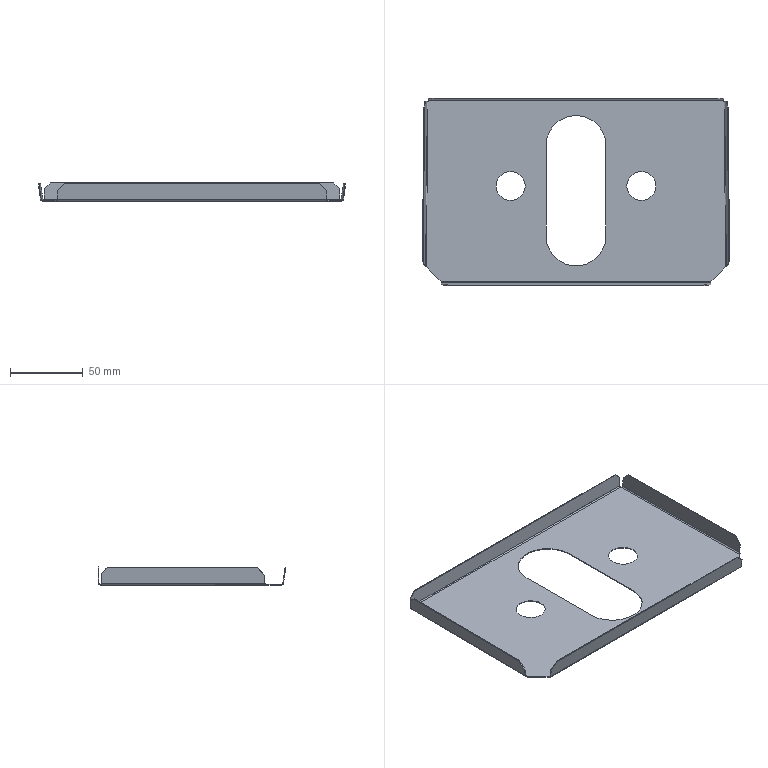Part | SolidWorks | features BaseBody 1 | 1 solid | 58 faces | box 211.542 x 129.145 x 12.429 mm | volume 14309 mm3 | plane 38 | cylinder 14 | spline 6 | commonest cylinder face diameters 1.5 x4 2.5 x4 20 x4 41.2 x2